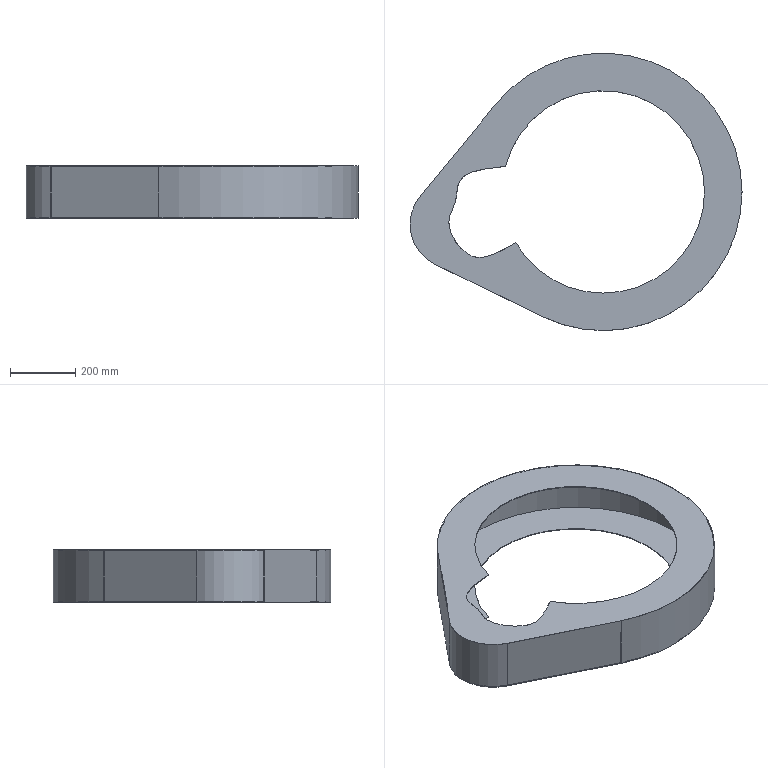Part | SolidWorks | features BaseBody 1 | 1 solid | 20 faces | box 1017 x 850 x 160 mm | volume 2046242 mm3 | cylinder 10 | plane 8 | spline 2 | commonest cylinder face diameters 620 x4 846 x2 850 x2 266 x1 270 x1